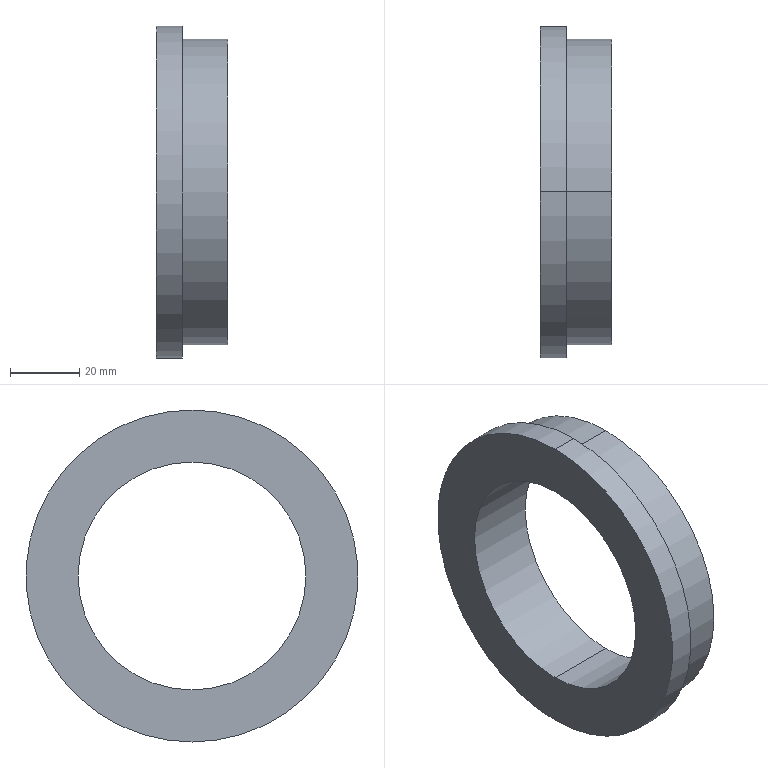Part | SolidWorks | features Revolution 1, Scale 1 | 1 solid | 9 faces | box 20.625 x 95.625 x 95.625 mm | volume 64156 mm3 | cylinder 6 | plane 3 | commonest cylinder face diameters 65.625 x2 88.125 x2 95.625 x2
STEP:
#1=CARTESIAN_POINT('',(-11.654,0.,-47.812));
#2=VERTEX_POINT('',#1);
#3=CARTESIAN_POINT('',(-11.654,0.,47.812));
#4=VERTEX_POINT('',#3);
#5=CARTESIAN_POINT('',(-11.654,0.,0.));
#6=DIRECTION('',(1.,0.,0.));
#7=DIRECTION('',(0.,0.,-1.));
#8=AXIS2_PLACEMENT_3D('',#5,#6,#7);
#9=CIRCLE('',#8,47.812);
#10=EDGE_CURVE('',#2,#4,#9,.T.);
#11=ORIENTED_EDGE('',*,*,#10,.T.);
#12=CARTESIAN_POINT('',(-4.154,0.,47.812));
#13=VERTEX_POINT('',#12);
#14=CARTESIAN_POINT('',(1.9,0.,47.812));
#15=DIRECTION('',(1.,0.,0.));
#16=VECTOR('',#15,1000.);
#17=LINE('',#14,#16);
#18=EDGE_CURVE('',#4,#13,#17,.T.);
#19=ORIENTED_EDGE('',*,*,#18,.T.);
#20=CARTESIAN_POINT('',(-4.154,0.,-47.812));
#21=VERTEX_POINT('',#20);
#22=CARTESIAN_POINT('',(-4.154,0.,0.));
#23=DIRECTION('',(1.,0.,0.));
#24=DIRECTION('',(0.,0.,-1.));
#25=AXIS2_PLACEMENT_3D('',#22,#23,#24);
#26=CIRCLE('',#25,47.812);
#27=EDGE_CURVE('',#21,#13,#26,.T.);
#28=ORIENTED_EDGE('',*,*,#27,.F.);
#29=CARTESIAN_POINT('',(1.9,0.,-47.812));
#30=DIRECTION('',(1.,0.,0.));
#31=VECTOR('',#30,1000.);
#32=LINE('',#29,#31);
#33=EDGE_CURVE('',#2,#21,#32,.T.);
#34=ORIENTED_EDGE('',*,*,#33,.F.);
#35=EDGE_LOOP('',(#11,#19,#28,#34));
#36=FACE_OUTER_BOUND('',#35,.T.);
#37=CARTESIAN_POINT('',(1.9,0.,0.));
#38=DIRECTION('',(1.,0.,0.));
#39=DIRECTION('',(0.,0.,-1.));
#40=AXIS2_PLACEMENT_3D('',#37,#38,#39);
#41=CYLINDRICAL_SURFACE('',#40,47.812);
#42=ADVANCED_FACE('',(#36),#41,.T.);
#43=CARTESIAN_POINT('',(-4.154,0.,-44.062));
#44=VERTEX_POINT('',#43);
#45=CARTESIAN_POINT('',(-4.154,0.,44.062));
#46=VERTEX_POINT('',#45);
#47=CARTESIAN_POINT('',(-4.154,0.,0.));
#48=DIRECTION('',(1.,0.,0.));
#49=DIRECTION('',(0.,0.,-1.));
#50=AXIS2_PLACEMENT_3D('',#47,#48,#49);
#51=CIRCLE('',#50,44.062);
#52=EDGE_CURVE('',#44,#46,#51,.T.);
#53=ORIENTED_EDGE('',*,*,#52,.T.);
#54=CARTESIAN_POINT('',(8.971,0.,44.062));
#55=VERTEX_POINT('',#54);
#56=CARTESIAN_POINT('',(1.9,0.,44.062));
#57=DIRECTION('',(1.,0.,0.));
#58=VECTOR('',#57,1000.);
#59=LINE('',#56,#58);
#60=EDGE_CURVE('',#46,#55,#59,.T.);
#61=ORIENTED_EDGE('',*,*,#60,.T.);
#62=CARTESIAN_POINT('',(8.971,0.,-44.062));
#63=VERTEX_POINT('',#62);
#64=CARTESIAN_POINT('',(8.971,0.,0.));
#65=DIRECTION('',(1.,0.,0.));
#66=DIRECTION('',(0.,0.,-1.));
#67=AXIS2_PLACEMENT_3D('',#64,#65,#66);
#68=CIRCLE('',#67,44.062);
#69=EDGE_CURVE('',#63,#55,#68,.T.);
#70=ORIENTED_EDGE('',*,*,#69,.F.);
#71=CARTESIAN_POINT('',(1.9,0.,-44.062));
#72=DIRECTION('',(1.,0.,0.));
#73=VECTOR('',#72,1000.);
#74=LINE('',#71,#73);
#75=EDGE_CURVE('',#44,#63,#74,.T.);
#76=ORIENTED_EDGE('',*,*,#75,.F.);
#77=EDGE_LOOP('',(#53,#61,#70,#76));
#78=FACE_OUTER_BOUND('',#77,.T.);
#79=CARTESIAN_POINT('',(1.9,0.,0.));
#80=DIRECTION('',(1.,0.,0.));
#81=DIRECTION('',(0.,0.,-1.));
#82=AXIS2_PLACEMENT_3D('',#79,#80,#81);
#83=CYLINDRICAL_SURFACE('',#82,44.062);
#84=ADVANCED_FACE('',(#78),#83,.T.);
#85=CARTESIAN_POINT('',(-11.654,0.,32.812));
#86=VERTEX_POINT('',#85);
#87=CARTESIAN_POINT('',(-11.654,0.,-32.812));
#88=VERTEX_POINT('',#87);
#89=CARTESIAN_POINT('',(-11.654,0.,0.));
#90=DIRECTION('',(1.,0.,0.));
#91=DIRECTION('',(0.,0.,-1.));
#92=AXIS2_PLACEMENT_3D('',#89,#90,#91);
#93=CIRCLE('',#92,32.812);
#94=EDGE_CURVE('',#86,#88,#93,.T.);
#95=ORIENTED_EDGE('',*,*,#94,.F.);
#96=CARTESIAN_POINT('',(8.971,0.,32.812));
#97=VERTEX_POINT('',#96);
#98=CARTESIAN_POINT('',(1.9,0.,32.812));
#99=DIRECTION('',(1.,0.,0.));
#100=VECTOR('',#99,1000.);
#101=LINE('',#98,#100);
#102=EDGE_CURVE('',#86,#97,#101,.T.);
#103=ORIENTED_EDGE('',*,*,#102,.T.);
#104=CARTESIAN_POINT('',(8.971,0.,-32.812));
#105=VERTEX_POINT('',#104);
#106=CARTESIAN_POINT('',(8.971,0.,0.));
#107=DIRECTION('',(1.,0.,0.));
#108=DIRECTION('',(0.,0.,-1.));
#109=AXIS2_PLACEMENT_3D('',#106,#107,#108);
#110=CIRCLE('',#109,32.812);
#111=EDGE_CURVE('',#97,#105,#110,.T.);
#112=ORIENTED_EDGE('',*,*,#111,.T.);
#113=CARTESIAN_POINT('',(1.9,0.,-32.812));
#114=DIRECTION('',(1.,0.,0.));
#115=VECTOR('',#114,1000.);
#116=LINE('',#113,#115);
#117=EDGE_CURVE('',#88,#105,#116,.T.);
#118=ORIENTED_EDGE('',*,*,#117,.F.);
#119=EDGE_LOOP('',(#95,#103,#112,#118));
#120=FACE_OUTER_BOUND('',#119,.T.);
#121=CARTESIAN_POINT('',(1.9,0.,0.));
#122=DIRECTION('',(1.,0.,0.));
#123=DIRECTION('',(0.,0.,-1.));
#124=AXIS2_PLACEMENT_3D('',#121,#122,#123);
#125=CYLINDRICAL_SURFACE('',#124,32.812);
#126=ADVANCED_FACE('',(#120),#125,.F.);
#127=CARTESIAN_POINT('',(-11.654,0.,0.));
#128=DIRECTION('',(1.,0.,0.));
#129=DIRECTION('',(0.,0.,-1.));
#130=AXIS2_PLACEMENT_3D('',#127,#128,#129);
#131=CIRCLE('',#130,32.812);
#132=EDGE_CURVE('',#88,#86,#131,.T.);
#133=ORIENTED_EDGE('',*,*,#132,.T.);
#134=ORIENTED_EDGE('',*,*,#94,.T.);
#135=EDGE_LOOP('',(#133,#134));
#136=FACE_BOUND('',#135,.T.);
#137=ORIENTED_EDGE('',*,*,#10,.F.);
#138=CARTESIAN_POINT('',(-11.654,0.,0.));
#139=DIRECTION('',(1.,0.,0.));
#140=DIRECTION('',(0.,0.,-1.));
#141=AXIS2_PLACEMENT_3D('',#138,#139,#140);
#142=CIRCLE('',#141,47.812);
#143=EDGE_CURVE('',#4,#2,#142,.T.);
#144=ORIENTED_EDGE('',*,*,#143,.F.);
#145=EDGE_LOOP('',(#137,#144));
#146=FACE_OUTER_BOUND('',#145,.T.);
#147=CARTESIAN_POINT('',(-11.654,47.812,0.));
#148=DIRECTION('',(-1.,0.,0.));
#149=DIRECTION('',(0.,0.,1.));
#150=AXIS2_PLACEMENT_3D('',#147,#148,#149);
#151=PLANE('',#150);
#152=ADVANCED_FACE('',(#136,#146),#151,.T.);
#153=ORIENTED_EDGE('',*,*,#102,.F.);
#154=ORIENTED_EDGE('',*,*,#132,.F.);
#155=ORIENTED_EDGE('',*,*,#117,.T.);
#156=CARTESIAN_POINT('',(8.971,0.,0.));
#157=DIRECTION('',(1.,0.,0.));
#158=DIRECTION('',(0.,0.,-1.));
#159=AXIS2_PLACEMENT_3D('',#156,#157,#158);
#160=CIRCLE('',#159,32.812);
#161=EDGE_CURVE('',#105,#97,#160,.T.);
#162=ORIENTED_EDGE('',*,*,#161,.T.);
#163=EDGE_LOOP('',(#153,#154,#155,#162));
#164=FACE_OUTER_BOUND('',#163,.T.);
#165=CARTESIAN_POINT('',(1.9,0.,0.));
#166=DIRECTION('',(1.,0.,0.));
#167=DIRECTION('',(0.,0.,-1.));
#168=AXIS2_PLACEMENT_3D('',#165,#166,#167);
#169=CYLINDRICAL_SURFACE('',#168,32.812);
#170=ADVANCED_FACE('',(#164),#169,.F.);
#171=ORIENTED_EDGE('',*,*,#69,.T.);
#172=CARTESIAN_POINT('',(8.971,0.,0.));
#173=DIRECTION('',(1.,0.,0.));
#174=DIRECTION('',(0.,0.,-1.));
#175=AXIS2_PLACEMENT_3D('',#172,#173,#174);
#176=CIRCLE('',#175,44.062);
#177=EDGE_CURVE('',#55,#63,#176,.T.);
#178=ORIENTED_EDGE('',*,*,#177,.T.);
#179=EDGE_LOOP('',(#171,#178));
#180=FACE_OUTER_BOUND('',#179,.T.);
#181=ORIENTED_EDGE('',*,*,#161,.F.);
#182=ORIENTED_EDGE('',*,*,#111,.F.);
#183=EDGE_LOOP('',(#181,#182));
#184=FACE_BOUND('',#183,.T.);
#185=CARTESIAN_POINT('',(8.971,32.812,0.));
#186=DIRECTION('',(1.,0.,0.));
#187=DIRECTION('',(0.,0.,-1.));
#188=AXIS2_PLACEMENT_3D('',#185,#186,#187);
#189=PLANE('',#188);
#190=ADVANCED_FACE('',(#180,#184),#189,.T.);
#191=ORIENTED_EDGE('',*,*,#60,.F.);
#192=CARTESIAN_POINT('',(-4.154,0.,0.));
#193=DIRECTION('',(1.,0.,0.));
#194=DIRECTION('',(0.,0.,-1.));
#195=AXIS2_PLACEMENT_3D('',#192,#193,#194);
#196=CIRCLE('',#195,44.062);
#197=EDGE_CURVE('',#46,#44,#196,.T.);
#198=ORIENTED_EDGE('',*,*,#197,.T.);
#199=ORIENTED_EDGE('',*,*,#75,.T.);
#200=ORIENTED_EDGE('',*,*,#177,.F.);
#201=EDGE_LOOP('',(#191,#198,#199,#200));
#202=FACE_OUTER_BOUND('',#201,.T.);
#203=CARTESIAN_POINT('',(1.9,0.,0.));
#204=DIRECTION('',(1.,0.,0.));
#205=DIRECTION('',(0.,0.,-1.));
#206=AXIS2_PLACEMENT_3D('',#203,#204,#205);
#207=CYLINDRICAL_SURFACE('',#206,44.062);
#208=ADVANCED_FACE('',(#202),#207,.T.);
#209=ORIENTED_EDGE('',*,*,#27,.T.);
#210=CARTESIAN_POINT('',(-4.154,0.,0.));
#211=DIRECTION('',(1.,0.,0.));
#212=DIRECTION('',(0.,0.,-1.));
#213=AXIS2_PLACEMENT_3D('',#210,#211,#212);
#214=CIRCLE('',#213,47.812);
#215=EDGE_CURVE('',#13,#21,#214,.T.);
#216=ORIENTED_EDGE('',*,*,#215,.T.);
#217=EDGE_LOOP('',(#209,#216));
#218=FACE_OUTER_BOUND('',#217,.T.);
#219=ORIENTED_EDGE('',*,*,#52,.F.);
#220=ORIENTED_EDGE('',*,*,#197,.F.);
#221=EDGE_LOOP('',(#219,#220));
#222=FACE_BOUND('',#221,.T.);
#223=CARTESIAN_POINT('',(-4.154,44.062,0.));
#224=DIRECTION('',(1.,0.,0.));
#225=DIRECTION('',(0.,0.,-1.));
#226=AXIS2_PLACEMENT_3D('',#223,#224,#225);
#227=PLANE('',#226);
#228=ADVANCED_FACE('',(#218,#222),#227,.T.);
#229=ORIENTED_EDGE('',*,*,#18,.F.);
#230=ORIENTED_EDGE('',*,*,#143,.T.);
#231=ORIENTED_EDGE('',*,*,#33,.T.);
#232=ORIENTED_EDGE('',*,*,#215,.F.);
#233=EDGE_LOOP('',(#229,#230,#231,#232));
#234=FACE_OUTER_BOUND('',#233,.T.);
#235=CARTESIAN_POINT('',(1.9,0.,0.));
#236=DIRECTION('',(1.,0.,0.));
#237=DIRECTION('',(0.,0.,-1.));
#238=AXIS2_PLACEMENT_3D('',#235,#236,#237);
#239=CYLINDRICAL_SURFACE('',#238,47.812);
#240=ADVANCED_FACE('',(#234),#239,.T.);
#241=CLOSED_SHELL('',(#42,#84,#126,#152,#170,#190,#208,#228,#240));
#242=MANIFOLD_SOLID_BREP('',#241);
#243=CARTESIAN_POINT('',(0.,0.,0.));
#244=DIRECTION('',(0.,0.,1.));
#245=DIRECTION('',(1.,0.,0.));
#246=AXIS2_PLACEMENT_3D('',#243,#244,#245);
#247=(LENGTH_UNIT()NAMED_UNIT(*)SI_UNIT(.MILLI.,.METRE.));
#248=UNCERTAINTY_MEASURE_WITH_UNIT(LENGTH_MEASURE(0.00001),#247,'','');
#249=(NAMED_UNIT(*)PLANE_ANGLE_UNIT()SI_UNIT($,.RADIAN.));
#250=(NAMED_UNIT(*)SI_UNIT($,.STERADIAN.)SOLID_ANGLE_UNIT());
#251=(GEOMETRIC_REPRESENTATION_CONTEXT(3)GLOBAL_UNCERTAINTY_ASSIGNED_CONTEXT((#248))GLOBAL_UNIT_ASSIGNED_CONTEXT((#247,#249,#250))REPRESENTATION_CONTEXT('',''));
#252=ADVANCED_BREP_SHAPE_REPRESENTATION('',(#242,#246),#251);